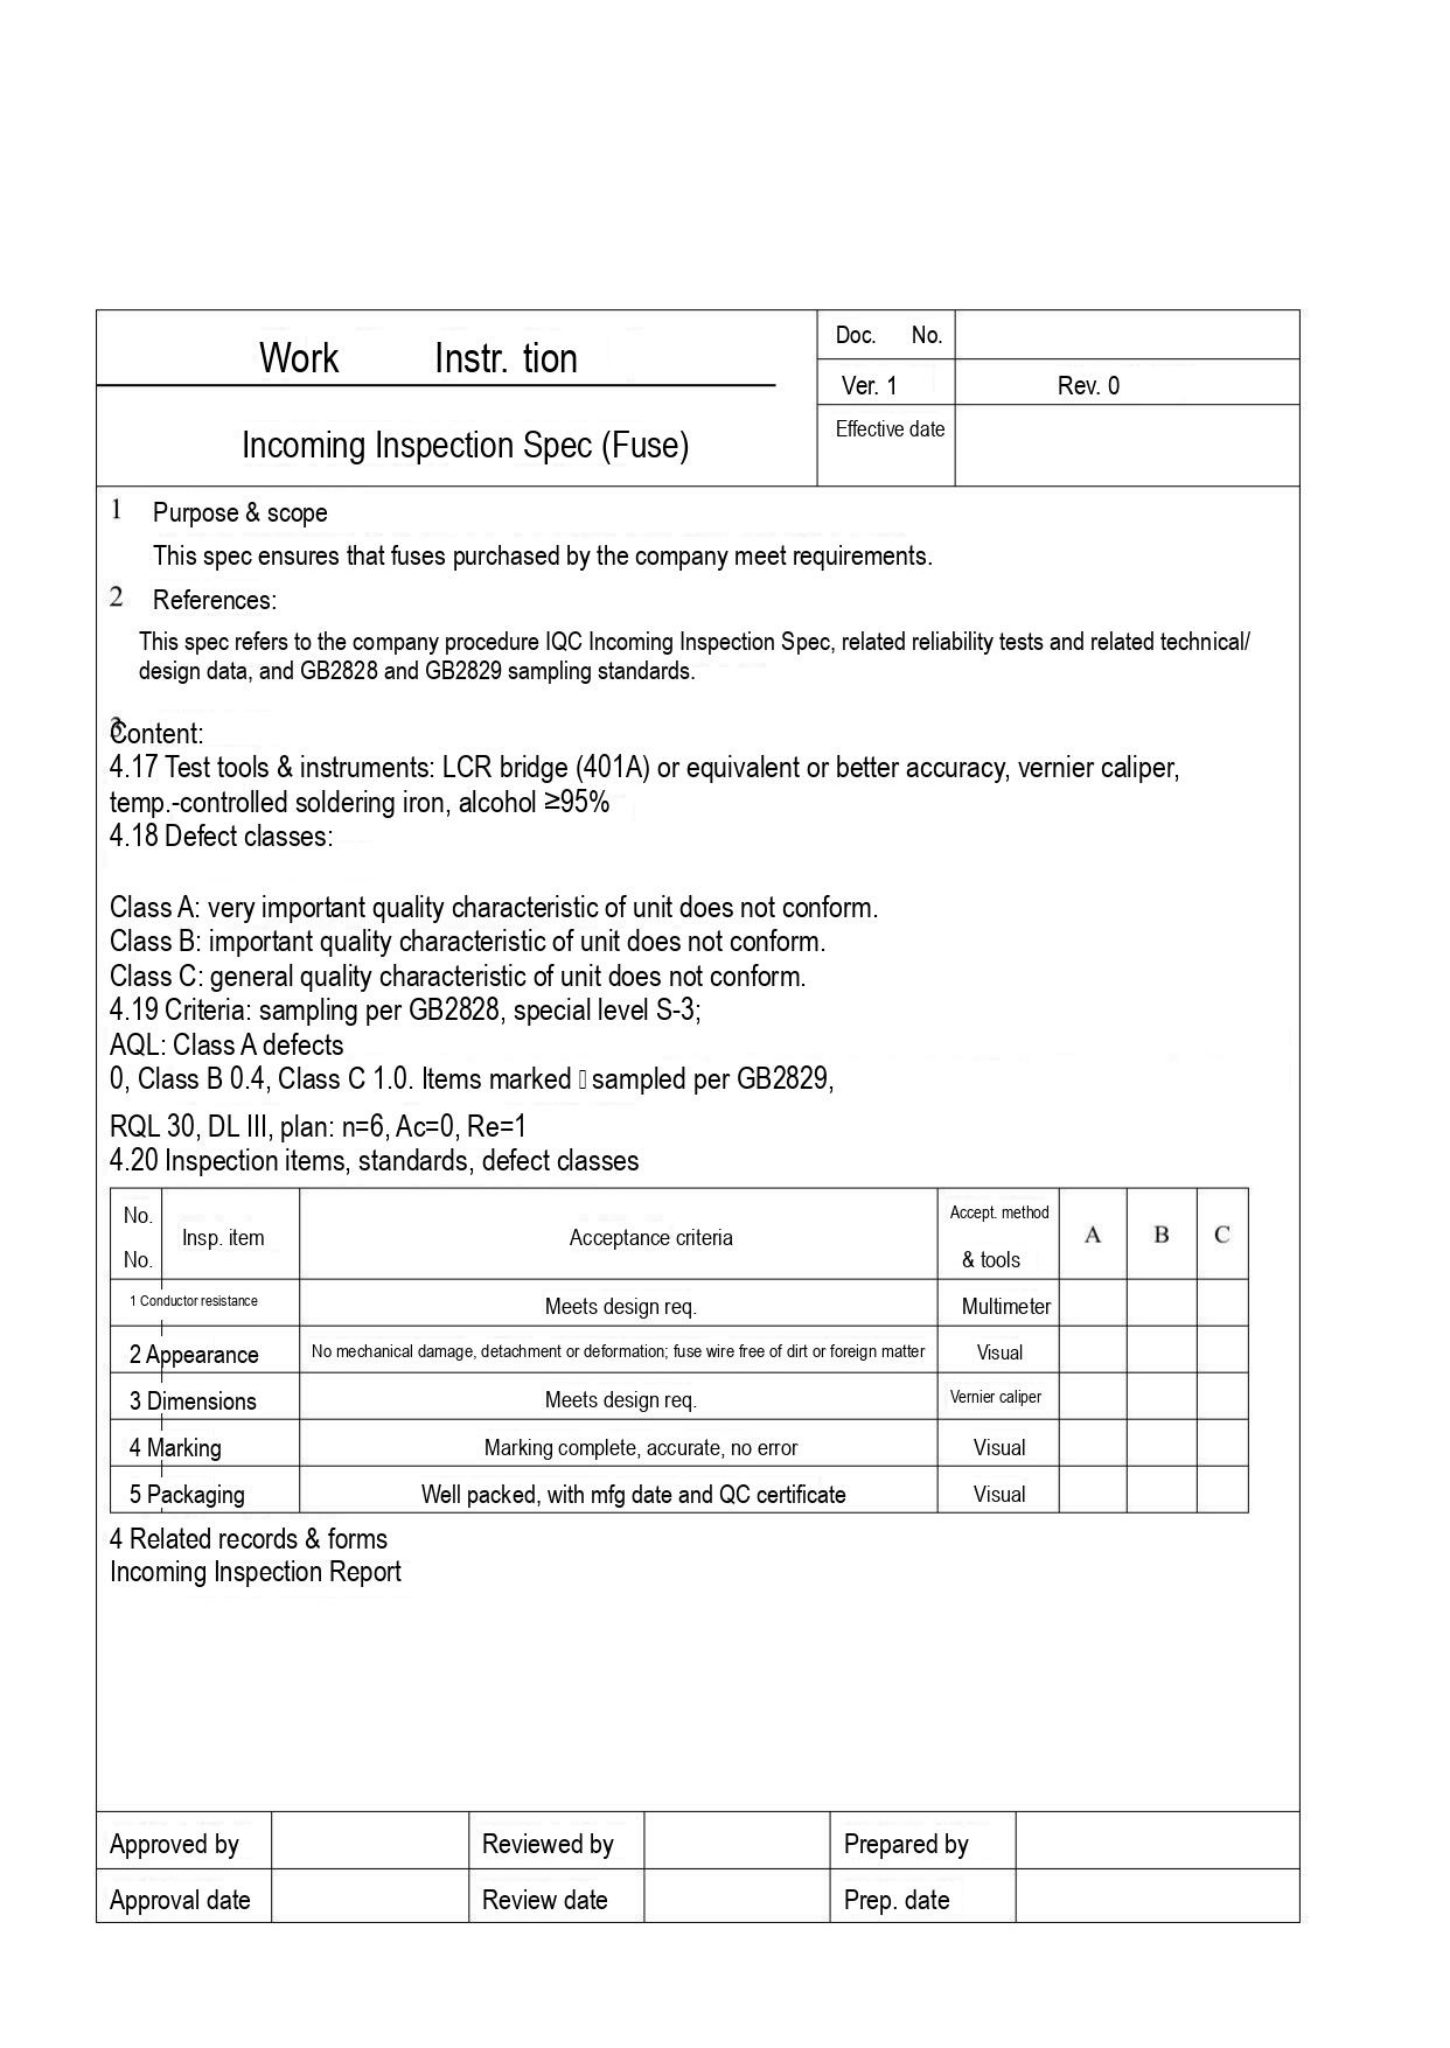| Work Instr. tion | Doc. No. | |
|---|---|---|
| | Ver. 1 | Rev. 0 |
| Incoming Inspection Spec (Fuse) | Effective date | |

1 Purpose & scope

This spec ensures that fuses purchased by the company meet requirements.

2 References:

This spec refers to the company procedure IQC Incoming Inspection Spec, related reliability tests and related technical/ design data, and GB2828 and GB2829 sampling standards.

Content:
4.17 Test tools & instruments: LCR bridge (401A) or equivalent or better accuracy, vernier caliper, temp.-controlled soldering iron, alcohol ≥95%
4.18 Defect classes:

Class A: very important quality characteristic of unit does not conform.
Class B: important quality characteristic of unit does not conform.
Class C: general quality characteristic of unit does not conform.
4.19 Criteria: sampling per GB2828, special level S-3;
AQL: Class A defects
0, Class B 0.4, Class C 1.0. Items marked sampled per GB2829,

RQL 30, DL III, plan: n=6, Ac=0, Re=1
4.20 Inspection items, standards, defect classes

| No. No. | Insp. item | Acceptance criteria | Accept. method & tools | A | B | C |
|---|---|---|---|---|---|---|
| 1 | Conductor resistance | Meets design req. | Multimeter | | | |
| 2 | Appearance | No mechanical damage, detachment or deformation; fuse wire free of dirt or foreign matter | Visual | | | |
| 3 | Dimensions | Meets design req. | Vernier caliper | | | |
| 4 | Marking | Marking complete, accurate, no error | Visual | | | |
| 5 | Packaging | Well packed, with mfg date and QC certificate | Visual | | | |

4 Related records & forms
Incoming Inspection Report

| Approved by | | Reviewed by | | Prepared by | |
|---|---|---|---|---|---|
| Approval date | | Review date | | Prep. date | |